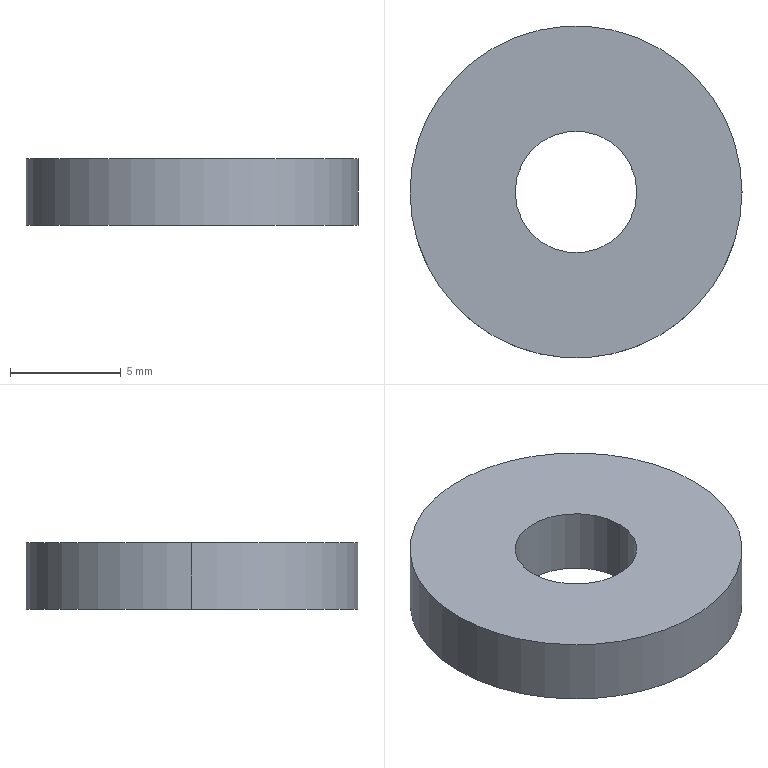Part | STEP file | locking washer | 1 solid | 6 faces | box 15 x 15 x 3 mm | volume 458.869 mm3 | cylinder 4 | plane 2 | commonest cylinder face diameters 5.5 x2 15 x2
STEP:
#1=CARTESIAN_POINT('',(0.,0.,0.));
#2=DIRECTION('',(0.,0.,1.));
#3=DIRECTION('',(1.,0.,0.));
#4=AXIS2_PLACEMENT_3D('',#1,#2,#3);
#5=CARTESIAN_POINT('',(-2.75,0.,3.));
#6=VERTEX_POINT('',#5);
#7=CARTESIAN_POINT('',(-2.75,0.,0.));
#8=VERTEX_POINT('',#7);
#9=CARTESIAN_POINT('',(-2.75,0.,3.));
#10=DIRECTION('',(0.,0.,-1.));
#11=VECTOR('',#10,1.);
#12=LINE('',#9,#11);
#13=CARTESIAN_POINT('',(0.,0.,3.));
#14=DIRECTION('',(0.,0.,-1.));
#15=DIRECTION('',(-1.,0.,0.));
#16=AXIS2_PLACEMENT_3D('',#13,#14,#15);
#17=CYLINDRICAL_SURFACE('',#16,2.75);
#18=CARTESIAN_POINT('',(6.283,0.));
#19=DIRECTION('',(0.,1.));
#20=VECTOR('',#19,1.);
#21=LINE('',#18,#20);
#22=(GEOMETRIC_REPRESENTATION_CONTEXT(2)PARAMETRIC_REPRESENTATION_CONTEXT()REPRESENTATION_CONTEXT('',''));
#23=DEFINITIONAL_REPRESENTATION('',(#21),#22);
#24=PCURVE('',#17,#23);
#25=CARTESIAN_POINT('',(0.,0.,3.));
#26=DIRECTION('',(0.,0.,-1.));
#27=DIRECTION('',(-1.,0.,0.));
#28=AXIS2_PLACEMENT_3D('',#25,#26,#27);
#29=CYLINDRICAL_SURFACE('',#28,2.75);
#30=CARTESIAN_POINT('',(0.,0.));
#31=DIRECTION('',(0.,1.));
#32=VECTOR('',#31,1.);
#33=LINE('',#30,#32);
#34=(GEOMETRIC_REPRESENTATION_CONTEXT(2)PARAMETRIC_REPRESENTATION_CONTEXT()REPRESENTATION_CONTEXT('',''));
#35=DEFINITIONAL_REPRESENTATION('',(#33),#34);
#36=PCURVE('',#29,#35);
#37=SURFACE_CURVE('',#12,(#24,#36),.PCURVE_S1.);
#38=EDGE_CURVE('',#6,#8,#37,.T.);
#39=ORIENTED_EDGE('',*,*,#38,.T.);
#40=CARTESIAN_POINT('',(2.75,0.,0.));
#41=VERTEX_POINT('',#40);
#42=CARTESIAN_POINT('',(0.,0.,0.));
#43=DIRECTION('',(0.,0.,1.));
#44=DIRECTION('',(1.,0.,0.));
#45=AXIS2_PLACEMENT_3D('',#42,#43,#44);
#46=CIRCLE('',#45,2.75);
#47=CARTESIAN_POINT('',(9.425,3.));
#48=DIRECTION('',(-1.,0.));
#49=VECTOR('',#48,1.);
#50=LINE('',#47,#49);
#51=(GEOMETRIC_REPRESENTATION_CONTEXT(2)PARAMETRIC_REPRESENTATION_CONTEXT()REPRESENTATION_CONTEXT('',''));
#52=DEFINITIONAL_REPRESENTATION('',(#50),#51);
#53=PCURVE('',#17,#52);
#54=CARTESIAN_POINT('',(0.,0.,0.));
#55=DIRECTION('',(0.,0.,1.));
#56=DIRECTION('',(1.,0.,0.));
#57=AXIS2_PLACEMENT_3D('',#54,#55,#56);
#58=PLANE('',#57);
#59=CARTESIAN_POINT('',(0.,0.));
#60=DIRECTION('',(1.,0.));
#61=AXIS2_PLACEMENT_2D('',#59,#60);
#62=CIRCLE('',#61,2.75);
#63=(GEOMETRIC_REPRESENTATION_CONTEXT(2)PARAMETRIC_REPRESENTATION_CONTEXT()REPRESENTATION_CONTEXT('',''));
#64=DEFINITIONAL_REPRESENTATION('',(#62),#63);
#65=PCURVE('',#58,#64);
#66=SURFACE_CURVE('',#46,(#53,#65),.PCURVE_S1.);
#67=EDGE_CURVE('',#8,#41,#66,.T.);
#68=ORIENTED_EDGE('',*,*,#67,.T.);
#69=CARTESIAN_POINT('',(2.75,0.,3.));
#70=VERTEX_POINT('',#69);
#71=CARTESIAN_POINT('',(2.75,0.,3.));
#72=DIRECTION('',(0.,0.,-1.));
#73=VECTOR('',#72,1.);
#74=LINE('',#71,#73);
#75=CARTESIAN_POINT('',(3.142,0.));
#76=DIRECTION('',(0.,1.));
#77=VECTOR('',#76,1.);
#78=LINE('',#75,#77);
#79=(GEOMETRIC_REPRESENTATION_CONTEXT(2)PARAMETRIC_REPRESENTATION_CONTEXT()REPRESENTATION_CONTEXT('',''));
#80=DEFINITIONAL_REPRESENTATION('',(#78),#79);
#81=PCURVE('',#17,#80);
#82=CARTESIAN_POINT('',(3.142,0.));
#83=DIRECTION('',(0.,1.));
#84=VECTOR('',#83,1.);
#85=LINE('',#82,#84);
#86=(GEOMETRIC_REPRESENTATION_CONTEXT(2)PARAMETRIC_REPRESENTATION_CONTEXT()REPRESENTATION_CONTEXT('',''));
#87=DEFINITIONAL_REPRESENTATION('',(#85),#86);
#88=PCURVE('',#29,#87);
#89=SURFACE_CURVE('',#74,(#81,#88),.PCURVE_S1.);
#90=EDGE_CURVE('',#70,#41,#89,.T.);
#91=ORIENTED_EDGE('',*,*,#90,.F.);
#92=CARTESIAN_POINT('',(0.,0.,3.));
#93=DIRECTION('',(0.,0.,1.));
#94=DIRECTION('',(1.,0.,0.));
#95=AXIS2_PLACEMENT_3D('',#92,#93,#94);
#96=CIRCLE('',#95,2.75);
#97=CARTESIAN_POINT('',(9.425,0.));
#98=DIRECTION('',(-1.,0.));
#99=VECTOR('',#98,1.);
#100=LINE('',#97,#99);
#101=(GEOMETRIC_REPRESENTATION_CONTEXT(2)PARAMETRIC_REPRESENTATION_CONTEXT()REPRESENTATION_CONTEXT('',''));
#102=DEFINITIONAL_REPRESENTATION('',(#100),#101);
#103=PCURVE('',#17,#102);
#104=CARTESIAN_POINT('',(0.,0.,3.));
#105=DIRECTION('',(0.,0.,1.));
#106=DIRECTION('',(1.,0.,0.));
#107=AXIS2_PLACEMENT_3D('',#104,#105,#106);
#108=PLANE('',#107);
#109=CARTESIAN_POINT('',(0.,0.));
#110=DIRECTION('',(1.,0.));
#111=AXIS2_PLACEMENT_2D('',#109,#110);
#112=CIRCLE('',#111,2.75);
#113=(GEOMETRIC_REPRESENTATION_CONTEXT(2)PARAMETRIC_REPRESENTATION_CONTEXT()REPRESENTATION_CONTEXT('',''));
#114=DEFINITIONAL_REPRESENTATION('',(#112),#113);
#115=PCURVE('',#108,#114);
#116=SURFACE_CURVE('',#96,(#103,#115),.PCURVE_S1.);
#117=EDGE_CURVE('',#6,#70,#116,.T.);
#118=ORIENTED_EDGE('',*,*,#117,.F.);
#119=EDGE_LOOP('',(#39,#68,#91,#118));
#120=FACE_BOUND('',#119,.F.);
#121=ADVANCED_FACE('',(#120),#17,.F.);
#122=CARTESIAN_POINT('',(7.5,0.,3.));
#123=VERTEX_POINT('',#122);
#124=CARTESIAN_POINT('',(-7.5,0.,3.));
#125=VERTEX_POINT('',#124);
#126=CARTESIAN_POINT('',(0.,0.,3.));
#127=DIRECTION('',(0.,0.,1.));
#128=DIRECTION('',(1.,0.,0.));
#129=AXIS2_PLACEMENT_3D('',#126,#127,#128);
#130=CIRCLE('',#129,7.5);
#131=CARTESIAN_POINT('',(0.,0.,3.));
#132=DIRECTION('',(0.,0.,-1.));
#133=DIRECTION('',(-1.,0.,0.));
#134=AXIS2_PLACEMENT_3D('',#131,#132,#133);
#135=CYLINDRICAL_SURFACE('',#134,7.5);
#136=CARTESIAN_POINT('',(3.142,0.));
#137=DIRECTION('',(-1.,0.));
#138=VECTOR('',#137,1.);
#139=LINE('',#136,#138);
#140=(GEOMETRIC_REPRESENTATION_CONTEXT(2)PARAMETRIC_REPRESENTATION_CONTEXT()REPRESENTATION_CONTEXT('',''));
#141=DEFINITIONAL_REPRESENTATION('',(#139),#140);
#142=PCURVE('',#135,#141);
#143=CARTESIAN_POINT('',(0.,0.));
#144=DIRECTION('',(1.,0.));
#145=AXIS2_PLACEMENT_2D('',#143,#144);
#146=CIRCLE('',#145,7.5);
#147=(GEOMETRIC_REPRESENTATION_CONTEXT(2)PARAMETRIC_REPRESENTATION_CONTEXT()REPRESENTATION_CONTEXT('',''));
#148=DEFINITIONAL_REPRESENTATION('',(#146),#147);
#149=PCURVE('',#108,#148);
#150=SURFACE_CURVE('',#130,(#142,#149),.PCURVE_S1.);
#151=EDGE_CURVE('',#123,#125,#150,.T.);
#152=ORIENTED_EDGE('',*,*,#151,.F.);
#153=CARTESIAN_POINT('',(7.5,0.,0.));
#154=VERTEX_POINT('',#153);
#155=CARTESIAN_POINT('',(7.5,0.,3.));
#156=DIRECTION('',(0.,0.,-1.));
#157=VECTOR('',#156,1.);
#158=LINE('',#155,#157);
#159=CARTESIAN_POINT('',(3.142,0.));
#160=DIRECTION('',(0.,1.));
#161=VECTOR('',#160,1.);
#162=LINE('',#159,#161);
#163=(GEOMETRIC_REPRESENTATION_CONTEXT(2)PARAMETRIC_REPRESENTATION_CONTEXT()REPRESENTATION_CONTEXT('',''));
#164=DEFINITIONAL_REPRESENTATION('',(#162),#163);
#165=PCURVE('',#135,#164);
#166=CARTESIAN_POINT('',(0.,0.,3.));
#167=DIRECTION('',(0.,0.,-1.));
#168=DIRECTION('',(-1.,0.,0.));
#169=AXIS2_PLACEMENT_3D('',#166,#167,#168);
#170=CYLINDRICAL_SURFACE('',#169,7.5);
#171=CARTESIAN_POINT('',(3.142,0.));
#172=DIRECTION('',(0.,1.));
#173=VECTOR('',#172,1.);
#174=LINE('',#171,#173);
#175=(GEOMETRIC_REPRESENTATION_CONTEXT(2)PARAMETRIC_REPRESENTATION_CONTEXT()REPRESENTATION_CONTEXT('',''));
#176=DEFINITIONAL_REPRESENTATION('',(#174),#175);
#177=PCURVE('',#170,#176);
#178=SURFACE_CURVE('',#158,(#165,#177),.PCURVE_S1.);
#179=EDGE_CURVE('',#123,#154,#178,.T.);
#180=ORIENTED_EDGE('',*,*,#179,.T.);
#181=CARTESIAN_POINT('',(-7.5,0.,0.));
#182=VERTEX_POINT('',#181);
#183=CARTESIAN_POINT('',(0.,0.,0.));
#184=DIRECTION('',(0.,0.,1.));
#185=DIRECTION('',(1.,0.,0.));
#186=AXIS2_PLACEMENT_3D('',#183,#184,#185);
#187=CIRCLE('',#186,7.5);
#188=CARTESIAN_POINT('',(3.142,3.));
#189=DIRECTION('',(-1.,0.));
#190=VECTOR('',#189,1.);
#191=LINE('',#188,#190);
#192=(GEOMETRIC_REPRESENTATION_CONTEXT(2)PARAMETRIC_REPRESENTATION_CONTEXT()REPRESENTATION_CONTEXT('',''));
#193=DEFINITIONAL_REPRESENTATION('',(#191),#192);
#194=PCURVE('',#135,#193);
#195=CARTESIAN_POINT('',(0.,0.));
#196=DIRECTION('',(1.,0.));
#197=AXIS2_PLACEMENT_2D('',#195,#196);
#198=CIRCLE('',#197,7.5);
#199=(GEOMETRIC_REPRESENTATION_CONTEXT(2)PARAMETRIC_REPRESENTATION_CONTEXT()REPRESENTATION_CONTEXT('',''));
#200=DEFINITIONAL_REPRESENTATION('',(#198),#199);
#201=PCURVE('',#58,#200);
#202=SURFACE_CURVE('',#187,(#194,#201),.PCURVE_S1.);
#203=EDGE_CURVE('',#154,#182,#202,.T.);
#204=ORIENTED_EDGE('',*,*,#203,.T.);
#205=CARTESIAN_POINT('',(-7.5,0.,3.));
#206=DIRECTION('',(0.,0.,-1.));
#207=VECTOR('',#206,1.);
#208=LINE('',#205,#207);
#209=CARTESIAN_POINT('',(0.,0.));
#210=DIRECTION('',(0.,1.));
#211=VECTOR('',#210,1.);
#212=LINE('',#209,#211);
#213=(GEOMETRIC_REPRESENTATION_CONTEXT(2)PARAMETRIC_REPRESENTATION_CONTEXT()REPRESENTATION_CONTEXT('',''));
#214=DEFINITIONAL_REPRESENTATION('',(#212),#213);
#215=PCURVE('',#135,#214);
#216=CARTESIAN_POINT('',(6.283,0.));
#217=DIRECTION('',(0.,1.));
#218=VECTOR('',#217,1.);
#219=LINE('',#216,#218);
#220=(GEOMETRIC_REPRESENTATION_CONTEXT(2)PARAMETRIC_REPRESENTATION_CONTEXT()REPRESENTATION_CONTEXT('',''));
#221=DEFINITIONAL_REPRESENTATION('',(#219),#220);
#222=PCURVE('',#170,#221);
#223=SURFACE_CURVE('',#208,(#215,#222),.PCURVE_S1.);
#224=EDGE_CURVE('',#125,#182,#223,.T.);
#225=ORIENTED_EDGE('',*,*,#224,.F.);
#226=EDGE_LOOP('',(#152,#180,#204,#225));
#227=FACE_BOUND('',#226,.T.);
#228=ADVANCED_FACE('',(#227),#135,.T.);
#229=CARTESIAN_POINT('',(0.,0.,3.));
#230=DIRECTION('',(0.,0.,1.));
#231=DIRECTION('',(1.,0.,0.));
#232=AXIS2_PLACEMENT_3D('',#229,#230,#231);
#233=CIRCLE('',#232,7.5);
#234=CARTESIAN_POINT('',(0.,0.));
#235=DIRECTION('',(1.,0.));
#236=AXIS2_PLACEMENT_2D('',#234,#235);
#237=CIRCLE('',#236,7.5);
#238=(GEOMETRIC_REPRESENTATION_CONTEXT(2)PARAMETRIC_REPRESENTATION_CONTEXT()REPRESENTATION_CONTEXT('',''));
#239=DEFINITIONAL_REPRESENTATION('',(#237),#238);
#240=PCURVE('',#108,#239);
#241=CARTESIAN_POINT('',(9.425,0.));
#242=DIRECTION('',(-1.,0.));
#243=VECTOR('',#242,1.);
#244=LINE('',#241,#243);
#245=(GEOMETRIC_REPRESENTATION_CONTEXT(2)PARAMETRIC_REPRESENTATION_CONTEXT()REPRESENTATION_CONTEXT('',''));
#246=DEFINITIONAL_REPRESENTATION('',(#244),#245);
#247=PCURVE('',#170,#246);
#248=SURFACE_CURVE('',#233,(#240,#247),.PCURVE_S1.);
#249=EDGE_CURVE('',#125,#123,#248,.T.);
#250=ORIENTED_EDGE('',*,*,#249,.T.);
#251=ORIENTED_EDGE('',*,*,#151,.T.);
#252=EDGE_LOOP('',(#250,#251));
#253=FACE_BOUND('',#252,.T.);
#254=ORIENTED_EDGE('',*,*,#117,.F.);
#255=CARTESIAN_POINT('',(0.,0.,3.));
#256=DIRECTION('',(0.,0.,1.));
#257=DIRECTION('',(1.,0.,0.));
#258=AXIS2_PLACEMENT_3D('',#255,#256,#257);
#259=CIRCLE('',#258,2.75);
#260=CARTESIAN_POINT('',(0.,0.));
#261=DIRECTION('',(1.,0.));
#262=AXIS2_PLACEMENT_2D('',#260,#261);
#263=CIRCLE('',#262,2.75);
#264=(GEOMETRIC_REPRESENTATION_CONTEXT(2)PARAMETRIC_REPRESENTATION_CONTEXT()REPRESENTATION_CONTEXT('',''));
#265=DEFINITIONAL_REPRESENTATION('',(#263),#264);
#266=PCURVE('',#108,#265);
#267=CARTESIAN_POINT('',(3.142,0.));
#268=DIRECTION('',(-1.,0.));
#269=VECTOR('',#268,1.);
#270=LINE('',#267,#269);
#271=(GEOMETRIC_REPRESENTATION_CONTEXT(2)PARAMETRIC_REPRESENTATION_CONTEXT()REPRESENTATION_CONTEXT('',''));
#272=DEFINITIONAL_REPRESENTATION('',(#270),#271);
#273=PCURVE('',#29,#272);
#274=SURFACE_CURVE('',#259,(#266,#273),.PCURVE_S1.);
#275=EDGE_CURVE('',#70,#6,#274,.T.);
#276=ORIENTED_EDGE('',*,*,#275,.F.);
#277=EDGE_LOOP('',(#254,#276));
#278=FACE_BOUND('',#277,.T.);
#279=ADVANCED_FACE('',(#253,#278),#108,.T.);
#280=CARTESIAN_POINT('',(0.,0.,0.));
#281=DIRECTION('',(0.,0.,1.));
#282=DIRECTION('',(1.,0.,0.));
#283=AXIS2_PLACEMENT_3D('',#280,#281,#282);
#284=CIRCLE('',#283,7.5);
#285=CARTESIAN_POINT('',(0.,0.));
#286=DIRECTION('',(1.,0.));
#287=AXIS2_PLACEMENT_2D('',#285,#286);
#288=CIRCLE('',#287,7.5);
#289=(GEOMETRIC_REPRESENTATION_CONTEXT(2)PARAMETRIC_REPRESENTATION_CONTEXT()REPRESENTATION_CONTEXT('',''));
#290=DEFINITIONAL_REPRESENTATION('',(#288),#289);
#291=PCURVE('',#58,#290);
#292=CARTESIAN_POINT('',(9.425,3.));
#293=DIRECTION('',(-1.,0.));
#294=VECTOR('',#293,1.);
#295=LINE('',#292,#294);
#296=(GEOMETRIC_REPRESENTATION_CONTEXT(2)PARAMETRIC_REPRESENTATION_CONTEXT()REPRESENTATION_CONTEXT('',''));
#297=DEFINITIONAL_REPRESENTATION('',(#295),#296);
#298=PCURVE('',#170,#297);
#299=SURFACE_CURVE('',#284,(#291,#298),.PCURVE_S1.);
#300=EDGE_CURVE('',#182,#154,#299,.T.);
#301=ORIENTED_EDGE('',*,*,#300,.F.);
#302=ORIENTED_EDGE('',*,*,#203,.F.);
#303=EDGE_LOOP('',(#301,#302));
#304=FACE_BOUND('',#303,.T.);
#305=ORIENTED_EDGE('',*,*,#67,.T.);
#306=CARTESIAN_POINT('',(0.,0.,0.));
#307=DIRECTION('',(0.,0.,1.));
#308=DIRECTION('',(1.,0.,0.));
#309=AXIS2_PLACEMENT_3D('',#306,#307,#308);
#310=CIRCLE('',#309,2.75);
#311=CARTESIAN_POINT('',(0.,0.));
#312=DIRECTION('',(1.,0.));
#313=AXIS2_PLACEMENT_2D('',#311,#312);
#314=CIRCLE('',#313,2.75);
#315=(GEOMETRIC_REPRESENTATION_CONTEXT(2)PARAMETRIC_REPRESENTATION_CONTEXT()REPRESENTATION_CONTEXT('',''));
#316=DEFINITIONAL_REPRESENTATION('',(#314),#315);
#317=PCURVE('',#58,#316);
#318=CARTESIAN_POINT('',(3.142,3.));
#319=DIRECTION('',(-1.,0.));
#320=VECTOR('',#319,1.);
#321=LINE('',#318,#320);
#322=(GEOMETRIC_REPRESENTATION_CONTEXT(2)PARAMETRIC_REPRESENTATION_CONTEXT()REPRESENTATION_CONTEXT('',''));
#323=DEFINITIONAL_REPRESENTATION('',(#321),#322);
#324=PCURVE('',#29,#323);
#325=SURFACE_CURVE('',#310,(#317,#324),.PCURVE_S1.);
#326=EDGE_CURVE('',#41,#8,#325,.T.);
#327=ORIENTED_EDGE('',*,*,#326,.T.);
#328=EDGE_LOOP('',(#305,#327));
#329=FACE_BOUND('',#328,.T.);
#330=ADVANCED_FACE('',(#304,#329),#58,.F.);
#331=ORIENTED_EDGE('',*,*,#179,.F.);
#332=ORIENTED_EDGE('',*,*,#249,.F.);
#333=ORIENTED_EDGE('',*,*,#224,.T.);
#334=ORIENTED_EDGE('',*,*,#300,.T.);
#335=EDGE_LOOP('',(#331,#332,#333,#334));
#336=FACE_BOUND('',#335,.T.);
#337=ADVANCED_FACE('',(#336),#170,.T.);
#338=ORIENTED_EDGE('',*,*,#326,.T.);
#339=ORIENTED_EDGE('',*,*,#38,.F.);
#340=ORIENTED_EDGE('',*,*,#275,.F.);
#341=ORIENTED_EDGE('',*,*,#90,.T.);
#342=EDGE_LOOP('',(#338,#339,#340,#341));
#343=FACE_BOUND('',#342,.F.);
#344=ADVANCED_FACE('',(#343),#29,.F.);
#345=CLOSED_SHELL('',(#121,#228,#279,#330,#337,#344));
#346=MANIFOLD_SOLID_BREP('',#345);
#347=(LENGTH_UNIT()NAMED_UNIT(*)SI_UNIT(.MILLI.,.METRE.));
#348=UNCERTAINTY_MEASURE_WITH_UNIT(LENGTH_MEASURE(0.0000001),#347,'','');
#349=(NAMED_UNIT(*)PLANE_ANGLE_UNIT()SI_UNIT($,.RADIAN.));
#350=(NAMED_UNIT(*)SI_UNIT($,.STERADIAN.)SOLID_ANGLE_UNIT());
#351=(GEOMETRIC_REPRESENTATION_CONTEXT(3)GLOBAL_UNCERTAINTY_ASSIGNED_CONTEXT((#348))GLOBAL_UNIT_ASSIGNED_CONTEXT((#347,#349,#350))REPRESENTATION_CONTEXT('',''));
#352=ADVANCED_BREP_SHAPE_REPRESENTATION('',(#4,#346),#351);